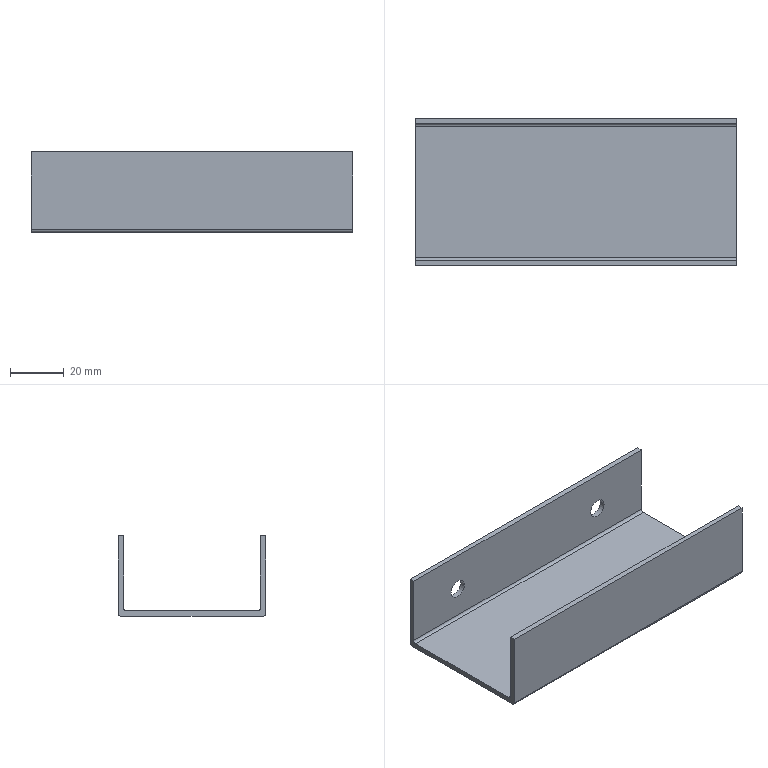Part | STEP file | 09-33 Motor support plate | 1 solid | 18 faces | box 120 x 55 x 30 mm | volume 26486 mm3 | plane 10 | cylinder 8 | commonest cylinder face diameters 2 x4 7 x4
STEP:
#1=CARTESIAN_POINT('',(0.,0.,0.));
#2=DIRECTION('',(0.,0.,1.));
#3=DIRECTION('',(1.,0.,0.));
#4=AXIS2_PLACEMENT_3D('',#1,#2,#3);
#5=CARTESIAN_POINT('',(33.27,53.,15.));
#6=VERTEX_POINT('',#5);
#7=CARTESIAN_POINT('',(33.27,55.,15.));
#8=VERTEX_POINT('',#7);
#9=CARTESIAN_POINT('',(33.27,53.,15.));
#10=DIRECTION('',(0.,1.,0.));
#11=VECTOR('',#10,1.);
#12=LINE('',#9,#11);
#13=CARTESIAN_POINT('',(36.77,53.,15.));
#14=DIRECTION('',(0.,1.,0.));
#15=DIRECTION('',(-1.,0.,0.));
#16=AXIS2_PLACEMENT_3D('',#13,#14,#15);
#17=CYLINDRICAL_SURFACE('',#16,3.5);
#18=CARTESIAN_POINT('',(6.283,0.));
#19=DIRECTION('',(0.,1.));
#20=VECTOR('',#19,1.);
#21=LINE('',#18,#20);
#22=(GEOMETRIC_REPRESENTATION_CONTEXT(2)PARAMETRIC_REPRESENTATION_CONTEXT()REPRESENTATION_CONTEXT('',''));
#23=DEFINITIONAL_REPRESENTATION('',(#21),#22);
#24=PCURVE('',#17,#23);
#25=CARTESIAN_POINT('',(36.77,53.,15.));
#26=DIRECTION('',(0.,1.,0.));
#27=DIRECTION('',(-1.,0.,0.));
#28=AXIS2_PLACEMENT_3D('',#25,#26,#27);
#29=CYLINDRICAL_SURFACE('',#28,3.5);
#30=CARTESIAN_POINT('',(0.,0.));
#31=DIRECTION('',(0.,1.));
#32=VECTOR('',#31,1.);
#33=LINE('',#30,#32);
#34=(GEOMETRIC_REPRESENTATION_CONTEXT(2)PARAMETRIC_REPRESENTATION_CONTEXT()REPRESENTATION_CONTEXT('',''));
#35=DEFINITIONAL_REPRESENTATION('',(#33),#34);
#36=PCURVE('',#29,#35);
#37=SURFACE_CURVE('',#12,(#24,#36),.PCURVE_S1.);
#38=EDGE_CURVE('',#6,#8,#37,.T.);
#39=ORIENTED_EDGE('',*,*,#38,.T.);
#40=CARTESIAN_POINT('',(40.27,55.,15.));
#41=VERTEX_POINT('',#40);
#42=CARTESIAN_POINT('',(36.77,55.,15.));
#43=DIRECTION('',(0.,1.,0.));
#44=DIRECTION('',(-1.,0.,0.));
#45=AXIS2_PLACEMENT_3D('',#42,#43,#44);
#46=CIRCLE('',#45,3.5);
#47=CARTESIAN_POINT('',(0.,2.));
#48=DIRECTION('',(1.,0.));
#49=VECTOR('',#48,1.);
#50=LINE('',#47,#49);
#51=(GEOMETRIC_REPRESENTATION_CONTEXT(2)PARAMETRIC_REPRESENTATION_CONTEXT()REPRESENTATION_CONTEXT('',''));
#52=DEFINITIONAL_REPRESENTATION('',(#50),#51);
#53=PCURVE('',#17,#52);
#54=CARTESIAN_POINT('',(-60.,55.,30.));
#55=DIRECTION('',(0.,-1.,0.));
#56=DIRECTION('',(0.,0.,-1.));
#57=AXIS2_PLACEMENT_3D('',#54,#55,#56);
#58=PLANE('',#57);
#59=CARTESIAN_POINT('',(15.,93.27));
#60=CARTESIAN_POINT('',(8.938,93.27));
#61=CARTESIAN_POINT('',(11.969,98.52));
#62=CARTESIAN_POINT('',(15.,103.77));
#63=CARTESIAN_POINT('',(18.031,98.52));
#64=CARTESIAN_POINT('',(21.062,93.27));
#65=CARTESIAN_POINT('',(15.,93.27));
#66=(BOUNDED_CURVE()B_SPLINE_CURVE(2,(#59,#60,#61,#62,#63,#64,#65),.UNSPECIFIED.,.T.,.F.)B_SPLINE_CURVE_WITH_KNOTS((1,2,2,2,2,1),(-2.094,0.,2.094,4.189,6.283,8.378),.UNSPECIFIED.)CURVE()GEOMETRIC_REPRESENTATION_ITEM()RATIONAL_B_SPLINE_CURVE((1.,0.5,1.,0.5,1.,0.5,1.))REPRESENTATION_ITEM(''));
#67=(GEOMETRIC_REPRESENTATION_CONTEXT(2)PARAMETRIC_REPRESENTATION_CONTEXT()REPRESENTATION_CONTEXT('',''));
#68=DEFINITIONAL_REPRESENTATION('',(#66),#67);
#69=PCURVE('',#58,#68);
#70=SURFACE_CURVE('',#46,(#53,#69),.PCURVE_S1.);
#71=EDGE_CURVE('',#41,#8,#70,.T.);
#72=ORIENTED_EDGE('',*,*,#71,.F.);
#73=CARTESIAN_POINT('',(40.27,53.,15.));
#74=VERTEX_POINT('',#73);
#75=CARTESIAN_POINT('',(40.27,53.,15.));
#76=DIRECTION('',(0.,1.,0.));
#77=VECTOR('',#76,1.);
#78=LINE('',#75,#77);
#79=CARTESIAN_POINT('',(3.142,0.));
#80=DIRECTION('',(0.,1.));
#81=VECTOR('',#80,1.);
#82=LINE('',#79,#81);
#83=(GEOMETRIC_REPRESENTATION_CONTEXT(2)PARAMETRIC_REPRESENTATION_CONTEXT()REPRESENTATION_CONTEXT('',''));
#84=DEFINITIONAL_REPRESENTATION('',(#82),#83);
#85=PCURVE('',#17,#84);
#86=CARTESIAN_POINT('',(3.142,0.));
#87=DIRECTION('',(0.,1.));
#88=VECTOR('',#87,1.);
#89=LINE('',#86,#88);
#90=(GEOMETRIC_REPRESENTATION_CONTEXT(2)PARAMETRIC_REPRESENTATION_CONTEXT()REPRESENTATION_CONTEXT('',''));
#91=DEFINITIONAL_REPRESENTATION('',(#89),#90);
#92=PCURVE('',#29,#91);
#93=SURFACE_CURVE('',#78,(#85,#92),.PCURVE_S1.);
#94=EDGE_CURVE('',#74,#41,#93,.T.);
#95=ORIENTED_EDGE('',*,*,#94,.F.);
#96=CARTESIAN_POINT('',(36.77,53.,15.));
#97=DIRECTION('',(0.,-1.,0.));
#98=DIRECTION('',(-1.,0.,0.));
#99=AXIS2_PLACEMENT_3D('',#96,#97,#98);
#100=CIRCLE('',#99,3.5);
#101=CARTESIAN_POINT('',(6.283,0.));
#102=DIRECTION('',(-1.,0.));
#103=VECTOR('',#102,1.);
#104=LINE('',#101,#103);
#105=(GEOMETRIC_REPRESENTATION_CONTEXT(2)PARAMETRIC_REPRESENTATION_CONTEXT()REPRESENTATION_CONTEXT('',''));
#106=DEFINITIONAL_REPRESENTATION('',(#104),#105);
#107=PCURVE('',#17,#106);
#108=CARTESIAN_POINT('',(-60.,53.,3.));
#109=DIRECTION('',(0.,1.,0.));
#110=DIRECTION('',(0.,0.,1.));
#111=AXIS2_PLACEMENT_3D('',#108,#109,#110);
#112=PLANE('',#111);
#113=CARTESIAN_POINT('',(12.,93.27));
#114=CARTESIAN_POINT('',(5.938,93.27));
#115=CARTESIAN_POINT('',(8.969,98.52));
#116=CARTESIAN_POINT('',(12.,103.77));
#117=CARTESIAN_POINT('',(15.031,98.52));
#118=CARTESIAN_POINT('',(18.062,93.27));
#119=CARTESIAN_POINT('',(12.,93.27));
#120=(BOUNDED_CURVE()B_SPLINE_CURVE(2,(#113,#114,#115,#116,#117,#118,#119),.UNSPECIFIED.,.T.,.F.)B_SPLINE_CURVE_WITH_KNOTS((1,2,2,2,2,1),(-2.094,0.,2.094,4.189,6.283,8.378),.UNSPECIFIED.)CURVE()GEOMETRIC_REPRESENTATION_ITEM()RATIONAL_B_SPLINE_CURVE((1.,0.5,1.,0.5,1.,0.5,1.))REPRESENTATION_ITEM(''));
#121=(GEOMETRIC_REPRESENTATION_CONTEXT(2)PARAMETRIC_REPRESENTATION_CONTEXT()REPRESENTATION_CONTEXT('',''));
#122=DEFINITIONAL_REPRESENTATION('',(#120),#121);
#123=PCURVE('',#112,#122);
#124=SURFACE_CURVE('',#100,(#107,#123),.PCURVE_S1.);
#125=EDGE_CURVE('',#6,#74,#124,.T.);
#126=ORIENTED_EDGE('',*,*,#125,.F.);
#127=EDGE_LOOP('',(#39,#72,#95,#126));
#128=FACE_BOUND('',#127,.F.);
#129=ADVANCED_FACE('',(#128),#17,.F.);
#130=CARTESIAN_POINT('',(-40.27,53.,15.));
#131=VERTEX_POINT('',#130);
#132=CARTESIAN_POINT('',(-40.27,55.,15.));
#133=VERTEX_POINT('',#132);
#134=CARTESIAN_POINT('',(-40.27,53.,15.));
#135=DIRECTION('',(0.,1.,0.));
#136=VECTOR('',#135,1.);
#137=LINE('',#134,#136);
#138=CARTESIAN_POINT('',(-36.77,53.,15.));
#139=DIRECTION('',(0.,1.,0.));
#140=DIRECTION('',(-1.,0.,0.));
#141=AXIS2_PLACEMENT_3D('',#138,#139,#140);
#142=CYLINDRICAL_SURFACE('',#141,3.5);
#143=CARTESIAN_POINT('',(6.283,0.));
#144=DIRECTION('',(0.,1.));
#145=VECTOR('',#144,1.);
#146=LINE('',#143,#145);
#147=(GEOMETRIC_REPRESENTATION_CONTEXT(2)PARAMETRIC_REPRESENTATION_CONTEXT()REPRESENTATION_CONTEXT('',''));
#148=DEFINITIONAL_REPRESENTATION('',(#146),#147);
#149=PCURVE('',#142,#148);
#150=CARTESIAN_POINT('',(-36.77,53.,15.));
#151=DIRECTION('',(0.,1.,0.));
#152=DIRECTION('',(-1.,0.,0.));
#153=AXIS2_PLACEMENT_3D('',#150,#151,#152);
#154=CYLINDRICAL_SURFACE('',#153,3.5);
#155=CARTESIAN_POINT('',(0.,0.));
#156=DIRECTION('',(0.,1.));
#157=VECTOR('',#156,1.);
#158=LINE('',#155,#157);
#159=(GEOMETRIC_REPRESENTATION_CONTEXT(2)PARAMETRIC_REPRESENTATION_CONTEXT()REPRESENTATION_CONTEXT('',''));
#160=DEFINITIONAL_REPRESENTATION('',(#158),#159);
#161=PCURVE('',#154,#160);
#162=SURFACE_CURVE('',#137,(#149,#161),.PCURVE_S1.);
#163=EDGE_CURVE('',#131,#133,#162,.T.);
#164=ORIENTED_EDGE('',*,*,#163,.T.);
#165=CARTESIAN_POINT('',(-33.27,55.,15.));
#166=VERTEX_POINT('',#165);
#167=CARTESIAN_POINT('',(-36.77,55.,15.));
#168=DIRECTION('',(0.,1.,0.));
#169=DIRECTION('',(-1.,0.,0.));
#170=AXIS2_PLACEMENT_3D('',#167,#168,#169);
#171=CIRCLE('',#170,3.5);
#172=CARTESIAN_POINT('',(0.,2.));
#173=DIRECTION('',(1.,0.));
#174=VECTOR('',#173,1.);
#175=LINE('',#172,#174);
#176=(GEOMETRIC_REPRESENTATION_CONTEXT(2)PARAMETRIC_REPRESENTATION_CONTEXT()REPRESENTATION_CONTEXT('',''));
#177=DEFINITIONAL_REPRESENTATION('',(#175),#176);
#178=PCURVE('',#142,#177);
#179=CARTESIAN_POINT('',(15.,19.73));
#180=CARTESIAN_POINT('',(8.938,19.73));
#181=CARTESIAN_POINT('',(11.969,24.98));
#182=CARTESIAN_POINT('',(15.,30.23));
#183=CARTESIAN_POINT('',(18.031,24.98));
#184=CARTESIAN_POINT('',(21.062,19.73));
#185=CARTESIAN_POINT('',(15.,19.73));
#186=(BOUNDED_CURVE()B_SPLINE_CURVE(2,(#179,#180,#181,#182,#183,#184,#185),.UNSPECIFIED.,.T.,.F.)B_SPLINE_CURVE_WITH_KNOTS((1,2,2,2,2,1),(-2.094,0.,2.094,4.189,6.283,8.378),.UNSPECIFIED.)CURVE()GEOMETRIC_REPRESENTATION_ITEM()RATIONAL_B_SPLINE_CURVE((1.,0.5,1.,0.5,1.,0.5,1.))REPRESENTATION_ITEM(''));
#187=(GEOMETRIC_REPRESENTATION_CONTEXT(2)PARAMETRIC_REPRESENTATION_CONTEXT()REPRESENTATION_CONTEXT('',''));
#188=DEFINITIONAL_REPRESENTATION('',(#186),#187);
#189=PCURVE('',#58,#188);
#190=SURFACE_CURVE('',#171,(#178,#189),.PCURVE_S1.);
#191=EDGE_CURVE('',#166,#133,#190,.T.);
#192=ORIENTED_EDGE('',*,*,#191,.F.);
#193=CARTESIAN_POINT('',(-33.27,53.,15.));
#194=VERTEX_POINT('',#193);
#195=CARTESIAN_POINT('',(-33.27,53.,15.));
#196=DIRECTION('',(0.,1.,0.));
#197=VECTOR('',#196,1.);
#198=LINE('',#195,#197);
#199=CARTESIAN_POINT('',(3.142,0.));
#200=DIRECTION('',(0.,1.));
#201=VECTOR('',#200,1.);
#202=LINE('',#199,#201);
#203=(GEOMETRIC_REPRESENTATION_CONTEXT(2)PARAMETRIC_REPRESENTATION_CONTEXT()REPRESENTATION_CONTEXT('',''));
#204=DEFINITIONAL_REPRESENTATION('',(#202),#203);
#205=PCURVE('',#142,#204);
#206=CARTESIAN_POINT('',(3.142,0.));
#207=DIRECTION('',(0.,1.));
#208=VECTOR('',#207,1.);
#209=LINE('',#206,#208);
#210=(GEOMETRIC_REPRESENTATION_CONTEXT(2)PARAMETRIC_REPRESENTATION_CONTEXT()REPRESENTATION_CONTEXT('',''));
#211=DEFINITIONAL_REPRESENTATION('',(#209),#210);
#212=PCURVE('',#154,#211);
#213=SURFACE_CURVE('',#198,(#205,#212),.PCURVE_S1.);
#214=EDGE_CURVE('',#194,#166,#213,.T.);
#215=ORIENTED_EDGE('',*,*,#214,.F.);
#216=CARTESIAN_POINT('',(-36.77,53.,15.));
#217=DIRECTION('',(0.,-1.,0.));
#218=DIRECTION('',(-1.,0.,0.));
#219=AXIS2_PLACEMENT_3D('',#216,#217,#218);
#220=CIRCLE('',#219,3.5);
#221=CARTESIAN_POINT('',(6.283,0.));
#222=DIRECTION('',(-1.,0.));
#223=VECTOR('',#222,1.);
#224=LINE('',#221,#223);
#225=(GEOMETRIC_REPRESENTATION_CONTEXT(2)PARAMETRIC_REPRESENTATION_CONTEXT()REPRESENTATION_CONTEXT('',''));
#226=DEFINITIONAL_REPRESENTATION('',(#224),#225);
#227=PCURVE('',#142,#226);
#228=CARTESIAN_POINT('',(12.,19.73));
#229=CARTESIAN_POINT('',(5.938,19.73));
#230=CARTESIAN_POINT('',(8.969,24.98));
#231=CARTESIAN_POINT('',(12.,30.23));
#232=CARTESIAN_POINT('',(15.031,24.98));
#233=CARTESIAN_POINT('',(18.062,19.73));
#234=CARTESIAN_POINT('',(12.,19.73));
#235=(BOUNDED_CURVE()B_SPLINE_CURVE(2,(#228,#229,#230,#231,#232,#233,#234),.UNSPECIFIED.,.T.,.F.)B_SPLINE_CURVE_WITH_KNOTS((1,2,2,2,2,1),(-2.094,0.,2.094,4.189,6.283,8.378),.UNSPECIFIED.)CURVE()GEOMETRIC_REPRESENTATION_ITEM()RATIONAL_B_SPLINE_CURVE((1.,0.5,1.,0.5,1.,0.5,1.))REPRESENTATION_ITEM(''));
#236=(GEOMETRIC_REPRESENTATION_CONTEXT(2)PARAMETRIC_REPRESENTATION_CONTEXT()REPRESENTATION_CONTEXT('',''));
#237=DEFINITIONAL_REPRESENTATION('',(#235),#236);
#238=PCURVE('',#112,#237);
#239=SURFACE_CURVE('',#220,(#227,#238),.PCURVE_S1.);
#240=EDGE_CURVE('',#131,#194,#239,.T.);
#241=ORIENTED_EDGE('',*,*,#240,.F.);
#242=EDGE_LOOP('',(#164,#192,#215,#241));
#243=FACE_BOUND('',#242,.F.);
#244=ADVANCED_FACE('',(#243),#142,.F.);
#245=CARTESIAN_POINT('',(36.77,55.,15.));
#246=DIRECTION('',(0.,1.,0.));
#247=DIRECTION('',(-1.,0.,0.));
#248=AXIS2_PLACEMENT_3D('',#245,#246,#247);
#249=CIRCLE('',#248,3.5);
#250=CARTESIAN_POINT('',(0.,2.));
#251=DIRECTION('',(1.,0.));
#252=VECTOR('',#251,1.);
#253=LINE('',#250,#252);
#254=(GEOMETRIC_REPRESENTATION_CONTEXT(2)PARAMETRIC_REPRESENTATION_CONTEXT()REPRESENTATION_CONTEXT('',''));
#255=DEFINITIONAL_REPRESENTATION('',(#253),#254);
#256=PCURVE('',#29,#255);
#257=CARTESIAN_POINT('',(15.,93.27));
#258=CARTESIAN_POINT('',(8.938,93.27));
#259=CARTESIAN_POINT('',(11.969,98.52));
#260=CARTESIAN_POINT('',(15.,103.77));
#261=CARTESIAN_POINT('',(18.031,98.52));
#262=CARTESIAN_POINT('',(21.062,93.27));
#263=CARTESIAN_POINT('',(15.,93.27));
#264=(BOUNDED_CURVE()B_SPLINE_CURVE(2,(#257,#258,#259,#260,#261,#262,#263),.UNSPECIFIED.,.T.,.F.)B_SPLINE_CURVE_WITH_KNOTS((1,2,2,2,2,1),(-2.094,0.,2.094,4.189,6.283,8.378),.UNSPECIFIED.)CURVE()GEOMETRIC_REPRESENTATION_ITEM()RATIONAL_B_SPLINE_CURVE((1.,0.5,1.,0.5,1.,0.5,1.))REPRESENTATION_ITEM(''));
#265=(GEOMETRIC_REPRESENTATION_CONTEXT(2)PARAMETRIC_REPRESENTATION_CONTEXT()REPRESENTATION_CONTEXT('',''));
#266=DEFINITIONAL_REPRESENTATION('',(#264),#265);
#267=PCURVE('',#58,#266);
#268=SURFACE_CURVE('',#249,(#256,#267),.PCURVE_S1.);
#269=EDGE_CURVE('',#8,#41,#268,.T.);
#270=ORIENTED_EDGE('',*,*,#269,.F.);
#271=ORIENTED_EDGE('',*,*,#38,.F.);
#272=CARTESIAN_POINT('',(36.77,53.,15.));
#273=DIRECTION('',(0.,-1.,0.));
#274=DIRECTION('',(-1.,0.,0.));
#275=AXIS2_PLACEMENT_3D('',#272,#273,#274);
#276=CIRCLE('',#275,3.5);
#277=CARTESIAN_POINT('',(6.283,0.));
#278=DIRECTION('',(-1.,0.));
#279=VECTOR('',#278,1.);
#280=LINE('',#277,#279);
#281=(GEOMETRIC_REPRESENTATION_CONTEXT(2)PARAMETRIC_REPRESENTATION_CONTEXT()REPRESENTATION_CONTEXT('',''));
#282=DEFINITIONAL_REPRESENTATION('',(#280),#281);
#283=PCURVE('',#29,#282);
#284=CARTESIAN_POINT('',(12.,93.27));
#285=CARTESIAN_POINT('',(5.938,93.27));
#286=CARTESIAN_POINT('',(8.969,98.52));
#287=CARTESIAN_POINT('',(12.,103.77));
#288=CARTESIAN_POINT('',(15.031,98.52));
#289=CARTESIAN_POINT('',(18.062,93.27));
#290=CARTESIAN_POINT('',(12.,93.27));
#291=(BOUNDED_CURVE()B_SPLINE_CURVE(2,(#284,#285,#286,#287,#288,#289,#290),.UNSPECIFIED.,.T.,.F.)B_SPLINE_CURVE_WITH_KNOTS((1,2,2,2,2,1),(-2.094,0.,2.094,4.189,6.283,8.378),.UNSPECIFIED.)CURVE()GEOMETRIC_REPRESENTATION_ITEM()RATIONAL_B_SPLINE_CURVE((1.,0.5,1.,0.5,1.,0.5,1.))REPRESENTATION_ITEM(''));
#292=(GEOMETRIC_REPRESENTATION_CONTEXT(2)PARAMETRIC_REPRESENTATION_CONTEXT()REPRESENTATION_CONTEXT('',''));
#293=DEFINITIONAL_REPRESENTATION('',(#291),#292);
#294=PCURVE('',#112,#293);
#295=SURFACE_CURVE('',#276,(#283,#294),.PCURVE_S1.);
#296=EDGE_CURVE('',#74,#6,#295,.T.);
#297=ORIENTED_EDGE('',*,*,#296,.F.);
#298=ORIENTED_EDGE('',*,*,#94,.T.);
#299=EDGE_LOOP('',(#270,#271,#297,#298));
#300=FACE_BOUND('',#299,.F.);
#301=ADVANCED_FACE('',(#300),#29,.F.);
#302=CARTESIAN_POINT('',(-36.77,55.,15.));
#303=DIRECTION('',(0.,1.,0.));
#304=DIRECTION('',(-1.,0.,0.));
#305=AXIS2_PLACEMENT_3D('',#302,#303,#304);
#306=CIRCLE('',#305,3.5);
#307=CARTESIAN_POINT('',(15.,19.73));
#308=CARTESIAN_POINT('',(8.938,19.73));
#309=CARTESIAN_POINT('',(11.969,24.98));
#310=CARTESIAN_POINT('',(15.,30.23));
#311=CARTESIAN_POINT('',(18.031,24.98));
#312=CARTESIAN_POINT('',(21.062,19.73));
#313=CARTESIAN_POINT('',(15.,19.73));
#314=(BOUNDED_CURVE()B_SPLINE_CURVE(2,(#307,#308,#309,#310,#311,#312,#313),.UNSPECIFIED.,.T.,.F.)B_SPLINE_CURVE_WITH_KNOTS((1,2,2,2,2,1),(-2.094,0.,2.094,4.189,6.283,8.378),.UNSPECIFIED.)CURVE()GEOMETRIC_REPRESENTATION_ITEM()RATIONAL_B_SPLINE_CURVE((1.,0.5,1.,0.5,1.,0.5,1.))REPRESENTATION_ITEM(''));
#315=(GEOMETRIC_REPRESENTATION_CONTEXT(2)PARAMETRIC_REPRESENTATION_CONTEXT()REPRESENTATION_CONTEXT('',''));
#316=DEFINITIONAL_REPRESENTATION('',(#314),#315);
#317=PCURVE('',#58,#316);
#318=CARTESIAN_POINT('',(0.,2.));
#319=DIRECTION('',(1.,0.));
#320=VECTOR('',#319,1.);
#321=LINE('',#318,#320);
#322=(GEOMETRIC_REPRESENTATION_CONTEXT(2)PARAMETRIC_REPRESENTATION_CONTEXT()REPRESENTATION_CONTEXT('',''));
#323=DEFINITIONAL_REPRESENTATION('',(#321),#322);
#324=PCURVE('',#154,#323);
#325=SURFACE_CURVE('',#306,(#317,#324),.PCURVE_S1.);
#326=EDGE_CURVE('',#133,#166,#325,.T.);
#327=ORIENTED_EDGE('',*,*,#326,.F.);
#328=ORIENTED_EDGE('',*,*,#191,.F.);
#329=EDGE_LOOP('',(#327,#328));
#330=FACE_BOUND('',#329,.T.);
#331=ORIENTED_EDGE('',*,*,#269,.F.);
#332=ORIENTED_EDGE('',*,*,#71,.F.);
#333=EDGE_LOOP('',(#331,#332));
#334=FACE_BOUND('',#333,.T.);
#335=CARTESIAN_POINT('',(-60.,55.,1.));
#336=VERTEX_POINT('',#335);
#337=CARTESIAN_POINT('',(60.,55.,1.));
#338=VERTEX_POINT('',#337);
#339=CARTESIAN_POINT('',(0.,55.,1.));
#340=DIRECTION('',(1.,0.,0.));
#341=VECTOR('',#340,1.);
#342=LINE('',#339,#341);
#343=CARTESIAN_POINT('',(29.,60.));
#344=DIRECTION('',(0.,1.));
#345=VECTOR('',#344,1.);
#346=LINE('',#343,#345);
#347=(GEOMETRIC_REPRESENTATION_CONTEXT(2)PARAMETRIC_REPRESENTATION_CONTEXT()REPRESENTATION_CONTEXT('',''));
#348=DEFINITIONAL_REPRESENTATION('',(#346),#347);
#349=PCURVE('',#58,#348);
#350=CARTESIAN_POINT('',(60.,54.,1.));
#351=DIRECTION('',(-1.,0.,0.));
#352=DIRECTION('',(0.,-1.,0.));
#353=AXIS2_PLACEMENT_3D('',#350,#351,#352);
#354=CYLINDRICAL_SURFACE('',#353,1.);
#355=CARTESIAN_POINT('',(3.142,60.));
#356=DIRECTION('',(0.,-1.));
#357=VECTOR('',#356,1.);
#358=LINE('',#355,#357);
#359=(GEOMETRIC_REPRESENTATION_CONTEXT(2)PARAMETRIC_REPRESENTATION_CONTEXT()REPRESENTATION_CONTEXT('',''));
#360=DEFINITIONAL_REPRESENTATION('',(#358),#359);
#361=PCURVE('',#354,#360);
#362=SURFACE_CURVE('',#342,(#349,#361),.PCURVE_S1.);
#363=EDGE_CURVE('',#336,#338,#362,.T.);
#364=ORIENTED_EDGE('',*,*,#363,.F.);
#365=CARTESIAN_POINT('',(-60.,55.,30.));
#366=VERTEX_POINT('',#365);
#367=CARTESIAN_POINT('',(-60.,55.,15.5));
#368=DIRECTION('',(0.,0.,-1.));
#369=VECTOR('',#368,1.);
#370=LINE('',#367,#369);
#371=CARTESIAN_POINT('',(14.5,0.));
#372=DIRECTION('',(1.,0.));
#373=VECTOR('',#372,1.);
#374=LINE('',#371,#373);
#375=(GEOMETRIC_REPRESENTATION_CONTEXT(2)PARAMETRIC_REPRESENTATION_CONTEXT()REPRESENTATION_CONTEXT('',''));
#376=DEFINITIONAL_REPRESENTATION('',(#374),#375);
#377=PCURVE('',#58,#376);
#378=CARTESIAN_POINT('',(-60.,0.,30.));
#379=DIRECTION('',(1.,0.,0.));
#380=DIRECTION('',(0.,0.,-1.));
#381=AXIS2_PLACEMENT_3D('',#378,#379,#380);
#382=PLANE('',#381);
#383=CARTESIAN_POINT('',(14.5,55.));
#384=DIRECTION('',(1.,0.));
#385=VECTOR('',#384,1.);
#386=LINE('',#383,#385);
#387=(GEOMETRIC_REPRESENTATION_CONTEXT(2)PARAMETRIC_REPRESENTATION_CONTEXT()REPRESENTATION_CONTEXT('',''));
#388=DEFINITIONAL_REPRESENTATION('',(#386),#387);
#389=PCURVE('',#382,#388);
#390=SURFACE_CURVE('',#370,(#377,#389),.PCURVE_S1.);
#391=EDGE_CURVE('',#366,#336,#390,.T.);
#392=ORIENTED_EDGE('',*,*,#391,.F.);
#393=CARTESIAN_POINT('',(60.,55.,30.));
#394=VERTEX_POINT('',#393);
#395=CARTESIAN_POINT('',(0.,55.,30.));
#396=DIRECTION('',(-1.,0.,0.));
#397=VECTOR('',#396,1.);
#398=LINE('',#395,#397);
#399=CARTESIAN_POINT('',(0.,60.));
#400=DIRECTION('',(0.,-1.));
#401=VECTOR('',#400,1.);
#402=LINE('',#399,#401);
#403=(GEOMETRIC_REPRESENTATION_CONTEXT(2)PARAMETRIC_REPRESENTATION_CONTEXT()REPRESENTATION_CONTEXT('',''));
#404=DEFINITIONAL_REPRESENTATION('',(#402),#403);
#405=PCURVE('',#58,#404);
#406=CARTESIAN_POINT('',(60.,53.,30.));
#407=DIRECTION('',(0.,0.,-1.));
#408=DIRECTION('',(-1.,0.,0.));
#409=AXIS2_PLACEMENT_3D('',#406,#407,#408);
#410=PLANE('',#409);
#411=CARTESIAN_POINT('',(60.,2.));
#412=DIRECTION('',(1.,0.));
#413=VECTOR('',#412,1.);
#414=LINE('',#411,#413);
#415=(GEOMETRIC_REPRESENTATION_CONTEXT(2)PARAMETRIC_REPRESENTATION_CONTEXT()REPRESENTATION_CONTEXT('',''));
#416=DEFINITIONAL_REPRESENTATION('',(#414),#415);
#417=PCURVE('',#410,#416);
#418=SURFACE_CURVE('',#398,(#405,#417),.PCURVE_S1.);
#419=EDGE_CURVE('',#394,#366,#418,.T.);
#420=ORIENTED_EDGE('',*,*,#419,.F.);
#421=CARTESIAN_POINT('',(60.,55.,15.5));
#422=DIRECTION('',(0.,0.,1.));
#423=VECTOR('',#422,1.);
#424=LINE('',#421,#423);
#425=CARTESIAN_POINT('',(14.5,120.));
#426=DIRECTION('',(-1.,0.));
#427=VECTOR('',#426,1.);
#428=LINE('',#425,#427);
#429=(GEOMETRIC_REPRESENTATION_CONTEXT(2)PARAMETRIC_REPRESENTATION_CONTEXT()REPRESENTATION_CONTEXT('',''));
#430=DEFINITIONAL_REPRESENTATION('',(#428),#429);
#431=PCURVE('',#58,#430);
#432=CARTESIAN_POINT('',(60.,0.,30.));
#433=DIRECTION('',(1.,0.,0.));
#434=DIRECTION('',(0.,0.,-1.));
#435=AXIS2_PLACEMENT_3D('',#432,#433,#434);
#436=PLANE('',#435);
#437=CARTESIAN_POINT('',(14.5,55.));
#438=DIRECTION('',(-1.,0.));
#439=VECTOR('',#438,1.);
#440=LINE('',#437,#439);
#441=(GEOMETRIC_REPRESENTATION_CONTEXT(2)PARAMETRIC_REPRESENTATION_CONTEXT()REPRESENTATION_CONTEXT('',''));
#442=DEFINITIONAL_REPRESENTATION('',(#440),#441);
#443=PCURVE('',#436,#442);
#444=SURFACE_CURVE('',#424,(#431,#443),.PCURVE_S1.);
#445=EDGE_CURVE('',#338,#394,#444,.T.);
#446=ORIENTED_EDGE('',*,*,#445,.F.);
#447=EDGE_LOOP('',(#364,#392,#420,#446));
#448=FACE_BOUND('',#447,.T.);
#449=ADVANCED_FACE('',(#330,#334,#448),#58,.F.);
#450=ORIENTED_EDGE('',*,*,#240,.F.);
#451=CARTESIAN_POINT('',(-36.77,53.,15.));
#452=DIRECTION('',(0.,-1.,0.));
#453=DIRECTION('',(-1.,0.,0.));
#454=AXIS2_PLACEMENT_3D('',#451,#452,#453);
#455=CIRCLE('',#454,3.5);
#456=CARTESIAN_POINT('',(12.,19.73));
#457=CARTESIAN_POINT('',(5.938,19.73));
#458=CARTESIAN_POINT('',(8.969,24.98));
#459=CARTESIAN_POINT('',(12.,30.23));
#460=CARTESIAN_POINT('',(15.031,24.98));
#461=CARTESIAN_POINT('',(18.062,19.73));
#462=CARTESIAN_POINT('',(12.,19.73));
#463=(BOUNDED_CURVE()B_SPLINE_CURVE(2,(#456,#457,#458,#459,#460,#461,#462),.UNSPECIFIED.,.T.,.F.)B_SPLINE_CURVE_WITH_KNOTS((1,2,2,2,2,1),(-2.094,0.,2.094,4.189,6.283,8.378),.UNSPECIFIED.)CURVE()GEOMETRIC_REPRESENTATION_ITEM()RATIONAL_B_SPLINE_CURVE((1.,0.5,1.,0.5,1.,0.5,1.))REPRESENTATION_ITEM(''));
#464=(GEOMETRIC_REPRESENTATION_CONTEXT(2)PARAMETRIC_REPRESENTATION_CONTEXT()REPRESENTATION_CONTEXT('',''));
#465=DEFINITIONAL_REPRESENTATION('',(#463),#464);
#466=PCURVE('',#112,#465);
#467=CARTESIAN_POINT('',(6.283,0.));
#468=DIRECTION('',(-1.,0.));
#469=VECTOR('',#468,1.);
#470=LINE('',#467,#469);
#471=(GEOMETRIC_REPRESENTATION_CONTEXT(2)PARAMETRIC_REPRESENTATION_CONTEXT()REPRESENTATION_CONTEXT('',''));
#472=DEFINITIONAL_REPRESENTATION('',(#470),#471);
#473=PCURVE('',#154,#472);
#474=SURFACE_CURVE('',#455,(#466,#473),.PCURVE_S1.);
#475=EDGE_CURVE('',#194,#131,#474,.T.);
#476=ORIENTED_EDGE('',*,*,#475,.F.);
#477=EDGE_LOOP('',(#450,#476));
#478=FACE_BOUND('',#477,.T.);
#479=ORIENTED_EDGE('',*,*,#125,.F.);
#480=ORIENTED_EDGE('',*,*,#296,.F.);
#481=EDGE_LOOP('',(#479,#480));
#482=FACE_BOUND('',#481,.T.);
#483=CARTESIAN_POINT('',(60.,53.,3.));
#484=VERTEX_POINT('',#483);
#485=CARTESIAN_POINT('',(-60.,53.,3.));
#486=VERTEX_POINT('',#485);
#487=CARTESIAN_POINT('',(0.,53.,3.));
#488=DIRECTION('',(-1.,0.,0.));
#489=VECTOR('',#488,1.);
#490=LINE('',#487,#489);
#491=CARTESIAN_POINT('',(0.,60.));
#492=DIRECTION('',(0.,-1.));
#493=VECTOR('',#492,1.);
#494=LINE('',#491,#493);
#495=(GEOMETRIC_REPRESENTATION_CONTEXT(2)PARAMETRIC_REPRESENTATION_CONTEXT()REPRESENTATION_CONTEXT('',''));
#496=DEFINITIONAL_REPRESENTATION('',(#494),#495);
#497=PCURVE('',#112,#496);
#498=CARTESIAN_POINT('',(-60.,52.,3.));
#499=DIRECTION('',(1.,0.,0.));
#500=DIRECTION('',(0.,1.,0.));
#501=AXIS2_PLACEMENT_3D('',#498,#499,#500);
#502=CYLINDRICAL_SURFACE('',#501,1.);
#503=CARTESIAN_POINT('',(6.283,60.));
#504=DIRECTION('',(0.,-1.));
#505=VECTOR('',#504,1.);
#506=LINE('',#503,#505);
#507=(GEOMETRIC_REPRESENTATION_CONTEXT(2)PARAMETRIC_REPRESENTATION_CONTEXT()REPRESENTATION_CONTEXT('',''));
#508=DEFINITIONAL_REPRESENTATION('',(#506),#507);
#509=PCURVE('',#502,#508);
#510=SURFACE_CURVE('',#490,(#497,#509),.PCURVE_S1.);
#511=EDGE_CURVE('',#484,#486,#510,.T.);
#512=ORIENTED_EDGE('',*,*,#511,.F.);
#513=CARTESIAN_POINT('',(60.,53.,30.));
#514=VERTEX_POINT('',#513);
#515=CARTESIAN_POINT('',(60.,53.,16.5));
#516=DIRECTION('',(0.,0.,-1.));
#517=VECTOR('',#516,1.);
#518=LINE('',#515,#517);
#519=CARTESIAN_POINT('',(13.5,120.));
#520=DIRECTION('',(-1.,0.));
#521=VECTOR('',#520,1.);
#522=LINE('',#519,#521);
#523=(GEOMETRIC_REPRESENTATION_CONTEXT(2)PARAMETRIC_REPRESENTATION_CONTEXT()REPRESENTATION_CONTEXT('',''));
#524=DEFINITIONAL_REPRESENTATION('',(#522),#523);
#525=PCURVE('',#112,#524);
#526=CARTESIAN_POINT('',(13.5,53.));
#527=DIRECTION('',(1.,0.));
#528=VECTOR('',#527,1.);
#529=LINE('',#526,#528);
#530=(GEOMETRIC_REPRESENTATION_CONTEXT(2)PARAMETRIC_REPRESENTATION_CONTEXT()REPRESENTATION_CONTEXT('',''));
#531=DEFINITIONAL_REPRESENTATION('',(#529),#530);
#532=PCURVE('',#436,#531);
#533=SURFACE_CURVE('',#518,(#525,#532),.PCURVE_S1.);
#534=EDGE_CURVE('',#514,#484,#533,.T.);
#535=ORIENTED_EDGE('',*,*,#534,.F.);
#536=CARTESIAN_POINT('',(-60.,53.,30.));
#537=VERTEX_POINT('',#536);
#538=CARTESIAN_POINT('',(0.,53.,30.));
#539=DIRECTION('',(1.,0.,0.));
#540=VECTOR('',#539,1.);
#541=LINE('',#538,#540);
#542=CARTESIAN_POINT('',(27.,60.));
#543=DIRECTION('',(0.,1.));
#544=VECTOR('',#543,1.);
#545=LINE('',#542,#544);
#546=(GEOMETRIC_REPRESENTATION_CONTEXT(2)PARAMETRIC_REPRESENTATION_CONTEXT()REPRESENTATION_CONTEXT('',''));
#547=DEFINITIONAL_REPRESENTATION('',(#545),#546);
#548=PCURVE('',#112,#547);
#549=CARTESIAN_POINT('',(60.,0.));
#550=DIRECTION('',(-1.,0.));
#551=VECTOR('',#550,1.);
#552=LINE('',#549,#551);
#553=(GEOMETRIC_REPRESENTATION_CONTEXT(2)PARAMETRIC_REPRESENTATION_CONTEXT()REPRESENTATION_CONTEXT('',''));
#554=DEFINITIONAL_REPRESENTATION('',(#552),#553);
#555=PCURVE('',#410,#554);
#556=SURFACE_CURVE('',#541,(#548,#555),.PCURVE_S1.);
#557=EDGE_CURVE('',#537,#514,#556,.T.);
#558=ORIENTED_EDGE('',*,*,#557,.F.);
#559=CARTESIAN_POINT('',(-60.,53.,16.5));
#560=DIRECTION('',(0.,0.,1.));
#561=VECTOR('',#560,1.);
#562=LINE('',#559,#561);
#563=CARTESIAN_POINT('',(13.5,0.));
#564=DIRECTION('',(1.,0.));
#565=VECTOR('',#564,1.);
#566=LINE('',#563,#565);
#567=(GEOMETRIC_REPRESENTATION_CONTEXT(2)PARAMETRIC_REPRESENTATION_CONTEXT()REPRESENTATION_CONTEXT('',''));
#568=DEFINITIONAL_REPRESENTATION('',(#566),#567);
#569=PCURVE('',#112,#568);
#570=CARTESIAN_POINT('',(13.5,53.));
#571=DIRECTION('',(-1.,0.));
#572=VECTOR('',#571,1.);
#573=LINE('',#570,#572);
#574=(GEOMETRIC_REPRESENTATION_CONTEXT(2)PARAMETRIC_REPRESENTATION_CONTEXT()REPRESENTATION_CONTEXT('',''));
#575=DEFINITIONAL_REPRESENTATION('',(#573),#574);
#576=PCURVE('',#382,#575);
#577=SURFACE_CURVE('',#562,(#569,#576),.PCURVE_S1.);
#578=EDGE_CURVE('',#486,#537,#577,.T.);
#579=ORIENTED_EDGE('',*,*,#578,.F.);
#580=EDGE_LOOP('',(#512,#535,#558,#579));
#581=FACE_BOUND('',#580,.T.);
#582=ADVANCED_FACE('',(#478,#482,#581),#112,.F.);
#583=ORIENTED_EDGE('',*,*,#326,.F.);
#584=ORIENTED_EDGE('',*,*,#163,.F.);
#585=ORIENTED_EDGE('',*,*,#475,.F.);
#586=ORIENTED_EDGE('',*,*,#214,.T.);
#587=EDGE_LOOP('',(#583,#584,#585,#586));
#588=FACE_BOUND('',#587,.F.);
#589=ADVANCED_FACE('',(#588),#154,.F.);
#590=CARTESIAN_POINT('',(60.,0.,30.));
#591=VERTEX_POINT('',#590);
#592=CARTESIAN_POINT('',(60.,0.,1.));
#593=VERTEX_POINT('',#592);
#594=CARTESIAN_POINT('',(60.,0.,15.));
#595=DIRECTION('',(0.,0.,-1.));
#596=VECTOR('',#595,1.);
#597=LINE('',#594,#596);
#598=CARTESIAN_POINT('',(15.,0.));
#599=DIRECTION('',(1.,0.));
#600=VECTOR('',#599,1.);
#601=LINE('',#598,#600);
#602=(GEOMETRIC_REPRESENTATION_CONTEXT(2)PARAMETRIC_REPRESENTATION_CONTEXT()REPRESENTATION_CONTEXT('',''));
#603=DEFINITIONAL_REPRESENTATION('',(#601),#602);
#604=PCURVE('',#436,#603);
#605=CARTESIAN_POINT('',(-60.,0.,1.));
#606=DIRECTION('',(0.,1.,0.));
#607=DIRECTION('',(0.,0.,1.));
#608=AXIS2_PLACEMENT_3D('',#605,#606,#607);
#609=PLANE('',#608);
#610=CARTESIAN_POINT('',(14.,120.));
#611=DIRECTION('',(-1.,0.));
#612=VECTOR('',#611,1.);
#613=LINE('',#610,#612);
#614=(GEOMETRIC_REPRESENTATION_CONTEXT(2)PARAMETRIC_REPRESENTATION_CONTEXT()REPRESENTATION_CONTEXT('',''));
#615=DEFINITIONAL_REPRESENTATION('',(#613),#614);
#616=PCURVE('',#609,#615);
#617=SURFACE_CURVE('',#597,(#604,#616),.PCURVE_S1.);
#618=EDGE_CURVE('',#591,#593,#617,.T.);
#619=ORIENTED_EDGE('',*,*,#618,.T.);
#620=CARTESIAN_POINT('',(60.,1.,0.));
#621=VERTEX_POINT('',#620);
#622=CARTESIAN_POINT('',(60.,1.,1.));
#623=DIRECTION('',(1.,0.,0.));
#624=DIRECTION('',(0.,-1.,0.));
#625=AXIS2_PLACEMENT_3D('',#622,#623,#624);
#626=CIRCLE('',#625,1.);
#627=CARTESIAN_POINT('',(29.,1.));
#628=DIRECTION('',(0.,-1.));
#629=AXIS2_PLACEMENT_2D('',#627,#628);
#630=CIRCLE('',#629,1.);
#631=(GEOMETRIC_REPRESENTATION_CONTEXT(2)PARAMETRIC_REPRESENTATION_CONTEXT()REPRESENTATION_CONTEXT('',''));
#632=DEFINITIONAL_REPRESENTATION('',(#630),#631);
#633=PCURVE('',#436,#632);
#634=CARTESIAN_POINT('',(60.,1.,1.));
#635=DIRECTION('',(-1.,0.,0.));
#636=DIRECTION('',(0.,-1.,0.));
#637=AXIS2_PLACEMENT_3D('',#634,#635,#636);
#638=CYLINDRICAL_SURFACE('',#637,1.);
#639=CARTESIAN_POINT('',(6.283,0.));
#640=DIRECTION('',(-1.,0.));
#641=VECTOR('',#640,1.);
#642=LINE('',#639,#641);
#643=(GEOMETRIC_REPRESENTATION_CONTEXT(2)PARAMETRIC_REPRESENTATION_CONTEXT()REPRESENTATION_CONTEXT('',''));
#644=DEFINITIONAL_REPRESENTATION('',(#642),#643);
#645=PCURVE('',#638,#644);
#646=SURFACE_CURVE('',#626,(#633,#645),.PCURVE_S1.);
#647=EDGE_CURVE('',#593,#621,#646,.T.);
#648=ORIENTED_EDGE('',*,*,#647,.T.);
#649=CARTESIAN_POINT('',(60.,54.,0.));
#650=VERTEX_POINT('',#649);
#651=CARTESIAN_POINT('',(60.,27.5,0.));
#652=DIRECTION('',(0.,1.,0.));
#653=VECTOR('',#652,1.);
#654=LINE('',#651,#653);
#655=CARTESIAN_POINT('',(30.,27.5));
#656=DIRECTION('',(0.,1.));
#657=VECTOR('',#656,1.);
#658=LINE('',#655,#657);
#659=(GEOMETRIC_REPRESENTATION_CONTEXT(2)PARAMETRIC_REPRESENTATION_CONTEXT()REPRESENTATION_CONTEXT('',''));
#660=DEFINITIONAL_REPRESENTATION('',(#658),#659);
#661=PCURVE('',#436,#660);
#662=CARTESIAN_POINT('',(-60.,1.,0.));
#663=DIRECTION('',(0.,0.,1.));
#664=DIRECTION('',(1.,0.,0.));
#665=AXIS2_PLACEMENT_3D('',#662,#663,#664);
#666=PLANE('',#665);
#667=CARTESIAN_POINT('',(120.,26.5));
#668=DIRECTION('',(0.,1.));
#669=VECTOR('',#668,1.);
#670=LINE('',#667,#669);
#671=(GEOMETRIC_REPRESENTATION_CONTEXT(2)PARAMETRIC_REPRESENTATION_CONTEXT()REPRESENTATION_CONTEXT('',''));
#672=DEFINITIONAL_REPRESENTATION('',(#670),#671);
#673=PCURVE('',#666,#672);
#674=SURFACE_CURVE('',#654,(#661,#673),.PCURVE_S1.);
#675=EDGE_CURVE('',#621,#650,#674,.T.);
#676=ORIENTED_EDGE('',*,*,#675,.T.);
#677=CARTESIAN_POINT('',(60.,54.,1.));
#678=DIRECTION('',(1.,0.,0.));
#679=DIRECTION('',(0.,-1.,0.));
#680=AXIS2_PLACEMENT_3D('',#677,#678,#679);
#681=CIRCLE('',#680,1.);
#682=CARTESIAN_POINT('',(29.,54.));
#683=DIRECTION('',(0.,-1.));
#684=AXIS2_PLACEMENT_2D('',#682,#683);
#685=CIRCLE('',#684,1.);
#686=(GEOMETRIC_REPRESENTATION_CONTEXT(2)PARAMETRIC_REPRESENTATION_CONTEXT()REPRESENTATION_CONTEXT('',''));
#687=DEFINITIONAL_REPRESENTATION('',(#685),#686);
#688=PCURVE('',#436,#687);
#689=CARTESIAN_POINT('',(6.283,0.));
#690=DIRECTION('',(-1.,0.));
#691=VECTOR('',#690,1.);
#692=LINE('',#689,#691);
#693=(GEOMETRIC_REPRESENTATION_CONTEXT(2)PARAMETRIC_REPRESENTATION_CONTEXT()REPRESENTATION_CONTEXT('',''));
#694=DEFINITIONAL_REPRESENTATION('',(#692),#693);
#695=PCURVE('',#354,#694);
#696=SURFACE_CURVE('',#681,(#688,#695),.PCURVE_S1.);
#697=EDGE_CURVE('',#650,#338,#696,.T.);
#698=ORIENTED_EDGE('',*,*,#697,.T.);
#699=ORIENTED_EDGE('',*,*,#445,.T.);
#700=CARTESIAN_POINT('',(60.,27.5,30.));
#701=DIRECTION('',(0.,-1.,0.));
#702=VECTOR('',#701,1.);
#703=LINE('',#700,#702);
#704=CARTESIAN_POINT('',(0.,27.5));
#705=DIRECTION('',(0.,-1.));
#706=VECTOR('',#705,1.);
#707=LINE('',#704,#706);
#708=(GEOMETRIC_REPRESENTATION_CONTEXT(2)PARAMETRIC_REPRESENTATION_CONTEXT()REPRESENTATION_CONTEXT('',''));
#709=DEFINITIONAL_REPRESENTATION('',(#707),#708);
#710=PCURVE('',#436,#709);
#711=CARTESIAN_POINT('',(0.,-25.5));
#712=DIRECTION('',(0.,-1.));
#713=VECTOR('',#712,1.);
#714=LINE('',#711,#713);
#715=(GEOMETRIC_REPRESENTATION_CONTEXT(2)PARAMETRIC_REPRESENTATION_CONTEXT()REPRESENTATION_CONTEXT('',''));
#716=DEFINITIONAL_REPRESENTATION('',(#714),#715);
#717=PCURVE('',#410,#716);
#718=SURFACE_CURVE('',#703,(#710,#717),.PCURVE_S1.);
#719=EDGE_CURVE('',#394,#514,#718,.T.);
#720=ORIENTED_EDGE('',*,*,#719,.T.);
#721=ORIENTED_EDGE('',*,*,#534,.T.);
#722=CARTESIAN_POINT('',(60.,52.,2.));
#723=VERTEX_POINT('',#722);
#724=CARTESIAN_POINT('',(60.,52.,3.));
#725=DIRECTION('',(-1.,0.,0.));
#726=DIRECTION('',(0.,1.,0.));
#727=AXIS2_PLACEMENT_3D('',#724,#725,#726);
#728=CIRCLE('',#727,1.);
#729=CARTESIAN_POINT('',(27.,53.));
#730=CARTESIAN_POINT('',(28.732,53.));
#731=CARTESIAN_POINT('',(27.866,51.5));
#732=CARTESIAN_POINT('',(27.,50.));
#733=CARTESIAN_POINT('',(26.134,51.5));
#734=CARTESIAN_POINT('',(25.268,53.));
#735=CARTESIAN_POINT('',(27.,53.));
#736=(BOUNDED_CURVE()B_SPLINE_CURVE(2,(#729,#730,#731,#732,#733,#734,#735),.UNSPECIFIED.,.T.,.F.)B_SPLINE_CURVE_WITH_KNOTS((1,2,2,2,2,1),(-2.094,0.,2.094,4.189,6.283,8.378),.UNSPECIFIED.)CURVE()GEOMETRIC_REPRESENTATION_ITEM()RATIONAL_B_SPLINE_CURVE((1.,0.5,1.,0.5,1.,0.5,1.))REPRESENTATION_ITEM(''));
#737=(GEOMETRIC_REPRESENTATION_CONTEXT(2)PARAMETRIC_REPRESENTATION_CONTEXT()REPRESENTATION_CONTEXT('',''));
#738=DEFINITIONAL_REPRESENTATION('',(#736),#737);
#739=PCURVE('',#436,#738);
#740=CARTESIAN_POINT('',(6.283,120.));
#741=DIRECTION('',(-1.,0.));
#742=VECTOR('',#741,1.);
#743=LINE('',#740,#742);
#744=(GEOMETRIC_REPRESENTATION_CONTEXT(2)PARAMETRIC_REPRESENTATION_CONTEXT()REPRESENTATION_CONTEXT('',''));
#745=DEFINITIONAL_REPRESENTATION('',(#743),#744);
#746=PCURVE('',#502,#745);
#747=SURFACE_CURVE('',#728,(#739,#746),.PCURVE_S1.);
#748=EDGE_CURVE('',#484,#723,#747,.T.);
#749=ORIENTED_EDGE('',*,*,#748,.T.);
#750=CARTESIAN_POINT('',(60.,3.,2.));
#751=VERTEX_POINT('',#750);
#752=CARTESIAN_POINT('',(60.,27.5,2.));
#753=DIRECTION('',(0.,-1.,0.));
#754=VECTOR('',#753,1.);
#755=LINE('',#752,#754);
#756=CARTESIAN_POINT('',(28.,27.5));
#757=DIRECTION('',(0.,-1.));
#758=VECTOR('',#757,1.);
#759=LINE('',#756,#758);
#760=(GEOMETRIC_REPRESENTATION_CONTEXT(2)PARAMETRIC_REPRESENTATION_CONTEXT()REPRESENTATION_CONTEXT('',''));
#761=DEFINITIONAL_REPRESENTATION('',(#759),#760);
#762=PCURVE('',#436,#761);
#763=CARTESIAN_POINT('',(-60.,3.,2.));
#764=DIRECTION('',(0.,0.,-1.));
#765=DIRECTION('',(0.,1.,0.));
#766=AXIS2_PLACEMENT_3D('',#763,#764,#765);
#767=PLANE('',#766);
#768=CARTESIAN_POINT('',(24.5,120.));
#769=DIRECTION('',(-1.,0.));
#770=VECTOR('',#769,1.);
#771=LINE('',#768,#770);
#772=(GEOMETRIC_REPRESENTATION_CONTEXT(2)PARAMETRIC_REPRESENTATION_CONTEXT()REPRESENTATION_CONTEXT('',''));
#773=DEFINITIONAL_REPRESENTATION('',(#771),#772);
#774=PCURVE('',#767,#773);
#775=SURFACE_CURVE('',#755,(#762,#774),.PCURVE_S1.);
#776=EDGE_CURVE('',#723,#751,#775,.T.);
#777=ORIENTED_EDGE('',*,*,#776,.T.);
#778=CARTESIAN_POINT('',(60.,2.,3.));
#779=VERTEX_POINT('',#778);
#780=CARTESIAN_POINT('',(60.,3.,3.));
#781=DIRECTION('',(1.,0.,0.));
#782=DIRECTION('',(0.,1.,0.));
#783=AXIS2_PLACEMENT_3D('',#780,#781,#782);
#784=CIRCLE('',#783,1.);
#785=CARTESIAN_POINT('',(27.,3.));
#786=DIRECTION('',(0.,1.));
#787=AXIS2_PLACEMENT_2D('',#785,#786);
#788=CIRCLE('',#787,1.);
#789=(GEOMETRIC_REPRESENTATION_CONTEXT(2)PARAMETRIC_REPRESENTATION_CONTEXT()REPRESENTATION_CONTEXT('',''));
#790=DEFINITIONAL_REPRESENTATION('',(#788),#789);
#791=PCURVE('',#436,#790);
#792=CARTESIAN_POINT('',(-60.,3.,3.));
#793=DIRECTION('',(1.,0.,0.));
#794=DIRECTION('',(0.,1.,0.));
#795=AXIS2_PLACEMENT_3D('',#792,#793,#794);
#796=CYLINDRICAL_SURFACE('',#795,1.);
#797=CARTESIAN_POINT('',(0.,120.));
#798=DIRECTION('',(1.,0.));
#799=VECTOR('',#798,1.);
#800=LINE('',#797,#799);
#801=(GEOMETRIC_REPRESENTATION_CONTEXT(2)PARAMETRIC_REPRESENTATION_CONTEXT()REPRESENTATION_CONTEXT('',''));
#802=DEFINITIONAL_REPRESENTATION('',(#800),#801);
#803=PCURVE('',#796,#802);
#804=SURFACE_CURVE('',#784,(#791,#803),.PCURVE_S1.);
#805=EDGE_CURVE('',#779,#751,#804,.T.);
#806=ORIENTED_EDGE('',*,*,#805,.F.);
#807=CARTESIAN_POINT('',(60.,2.,30.));
#808=VERTEX_POINT('',#807);
#809=CARTESIAN_POINT('',(60.,2.,15.));
#810=DIRECTION('',(0.,0.,1.));
#811=VECTOR('',#810,1.);
#812=LINE('',#809,#811);
#813=CARTESIAN_POINT('',(15.,2.));
#814=DIRECTION('',(-1.,0.));
#815=VECTOR('',#814,1.);
#816=LINE('',#813,#815);
#817=(GEOMETRIC_REPRESENTATION_CONTEXT(2)PARAMETRIC_REPRESENTATION_CONTEXT()REPRESENTATION_CONTEXT('',''));
#818=DEFINITIONAL_REPRESENTATION('',(#816),#817);
#819=PCURVE('',#436,#818);
#820=CARTESIAN_POINT('',(-60.,2.,30.));
#821=DIRECTION('',(0.,-1.,0.));
#822=DIRECTION('',(0.,0.,-1.));
#823=AXIS2_PLACEMENT_3D('',#820,#821,#822);
#824=PLANE('',#823);
#825=CARTESIAN_POINT('',(15.,120.));
#826=DIRECTION('',(-1.,0.));
#827=VECTOR('',#826,1.);
#828=LINE('',#825,#827);
#829=(GEOMETRIC_REPRESENTATION_CONTEXT(2)PARAMETRIC_REPRESENTATION_CONTEXT()REPRESENTATION_CONTEXT('',''));
#830=DEFINITIONAL_REPRESENTATION('',(#828),#829);
#831=PCURVE('',#824,#830);
#832=SURFACE_CURVE('',#812,(#819,#831),.PCURVE_S1.);
#833=EDGE_CURVE('',#779,#808,#832,.T.);
#834=ORIENTED_EDGE('',*,*,#833,.T.);
#835=CARTESIAN_POINT('',(60.,27.5,30.));
#836=DIRECTION('',(0.,-1.,0.));
#837=VECTOR('',#836,1.);
#838=LINE('',#835,#837);
#839=CARTESIAN_POINT('',(0.,27.5));
#840=DIRECTION('',(0.,-1.));
#841=VECTOR('',#840,1.);
#842=LINE('',#839,#841);
#843=(GEOMETRIC_REPRESENTATION_CONTEXT(2)PARAMETRIC_REPRESENTATION_CONTEXT()REPRESENTATION_CONTEXT('',''));
#844=DEFINITIONAL_REPRESENTATION('',(#842),#843);
#845=PCURVE('',#436,#844);
#846=CARTESIAN_POINT('',(60.,0.,30.));
#847=DIRECTION('',(0.,0.,-1.));
#848=DIRECTION('',(-1.,0.,0.));
#849=AXIS2_PLACEMENT_3D('',#846,#847,#848);
#850=PLANE('',#849);
#851=CARTESIAN_POINT('',(0.,27.5));
#852=DIRECTION('',(0.,-1.));
#853=VECTOR('',#852,1.);
#854=LINE('',#851,#853);
#855=(GEOMETRIC_REPRESENTATION_CONTEXT(2)PARAMETRIC_REPRESENTATION_CONTEXT()REPRESENTATION_CONTEXT('',''));
#856=DEFINITIONAL_REPRESENTATION('',(#854),#855);
#857=PCURVE('',#850,#856);
#858=SURFACE_CURVE('',#838,(#845,#857),.PCURVE_S1.);
#859=EDGE_CURVE('',#808,#591,#858,.T.);
#860=ORIENTED_EDGE('',*,*,#859,.T.);
#861=EDGE_LOOP('',(#619,#648,#676,#698,#699,#720,#721,#749,#777,#806,#834,#860));
#862=FACE_BOUND('',#861,.T.);
#863=ADVANCED_FACE('',(#862),#436,.T.);
#864=CARTESIAN_POINT('',(-60.,54.,0.));
#865=VERTEX_POINT('',#864);
#866=CARTESIAN_POINT('',(0.,54.,0.));
#867=DIRECTION('',(1.,0.,0.));
#868=VECTOR('',#867,1.);
#869=LINE('',#866,#868);
#870=CARTESIAN_POINT('',(4.712,60.));
#871=DIRECTION('',(0.,-1.));
#872=VECTOR('',#871,1.);
#873=LINE('',#870,#872);
#874=(GEOMETRIC_REPRESENTATION_CONTEXT(2)PARAMETRIC_REPRESENTATION_CONTEXT()REPRESENTATION_CONTEXT('',''));
#875=DEFINITIONAL_REPRESENTATION('',(#873),#874);
#876=PCURVE('',#354,#875);
#877=CARTESIAN_POINT('',(60.,53.));
#878=DIRECTION('',(1.,0.));
#879=VECTOR('',#878,1.);
#880=LINE('',#877,#879);
#881=(GEOMETRIC_REPRESENTATION_CONTEXT(2)PARAMETRIC_REPRESENTATION_CONTEXT()REPRESENTATION_CONTEXT('',''));
#882=DEFINITIONAL_REPRESENTATION('',(#880),#881);
#883=PCURVE('',#666,#882);
#884=SURFACE_CURVE('',#869,(#876,#883),.PCURVE_S1.);
#885=EDGE_CURVE('',#865,#650,#884,.T.);
#886=ORIENTED_EDGE('',*,*,#885,.F.);
#887=CARTESIAN_POINT('',(-60.,54.,1.));
#888=DIRECTION('',(-1.,0.,0.));
#889=DIRECTION('',(0.,-1.,0.));
#890=AXIS2_PLACEMENT_3D('',#887,#888,#889);
#891=CIRCLE('',#890,1.);
#892=CARTESIAN_POINT('',(0.,120.));
#893=DIRECTION('',(1.,0.));
#894=VECTOR('',#893,1.);
#895=LINE('',#892,#894);
#896=(GEOMETRIC_REPRESENTATION_CONTEXT(2)PARAMETRIC_REPRESENTATION_CONTEXT()REPRESENTATION_CONTEXT('',''));
#897=DEFINITIONAL_REPRESENTATION('',(#895),#896);
#898=PCURVE('',#354,#897);
#899=CARTESIAN_POINT('',(29.,53.));
#900=CARTESIAN_POINT('',(27.268,53.));
#901=CARTESIAN_POINT('',(28.134,54.5));
#902=CARTESIAN_POINT('',(29.,56.));
#903=CARTESIAN_POINT('',(29.866,54.5));
#904=CARTESIAN_POINT('',(30.732,53.));
#905=CARTESIAN_POINT('',(29.,53.));
#906=(BOUNDED_CURVE()B_SPLINE_CURVE(2,(#899,#900,#901,#902,#903,#904,#905),.UNSPECIFIED.,.T.,.F.)B_SPLINE_CURVE_WITH_KNOTS((1,2,2,2,2,1),(-2.094,0.,2.094,4.189,6.283,8.378),.UNSPECIFIED.)CURVE()GEOMETRIC_REPRESENTATION_ITEM()RATIONAL_B_SPLINE_CURVE((1.,0.5,1.,0.5,1.,0.5,1.))REPRESENTATION_ITEM(''));
#907=(GEOMETRIC_REPRESENTATION_CONTEXT(2)PARAMETRIC_REPRESENTATION_CONTEXT()REPRESENTATION_CONTEXT('',''));
#908=DEFINITIONAL_REPRESENTATION('',(#906),#907);
#909=PCURVE('',#382,#908);
#910=SURFACE_CURVE('',#891,(#898,#909),.PCURVE_S1.);
#911=EDGE_CURVE('',#336,#865,#910,.T.);
#912=ORIENTED_EDGE('',*,*,#911,.F.);
#913=ORIENTED_EDGE('',*,*,#363,.T.);
#914=ORIENTED_EDGE('',*,*,#697,.F.);
#915=EDGE_LOOP('',(#886,#912,#913,#914));
#916=FACE_BOUND('',#915,.T.);
#917=ADVANCED_FACE('',(#916),#354,.T.);
#918=ORIENTED_EDGE('',*,*,#911,.T.);
#919=CARTESIAN_POINT('',(-60.,1.,0.));
#920=VERTEX_POINT('',#919);
#921=CARTESIAN_POINT('',(-60.,27.5,0.));
#922=DIRECTION('',(0.,1.,0.));
#923=VECTOR('',#922,1.);
#924=LINE('',#921,#923);
#925=CARTESIAN_POINT('',(30.,27.5));
#926=DIRECTION('',(0.,1.));
#927=VECTOR('',#926,1.);
#928=LINE('',#925,#927);
#929=(GEOMETRIC_REPRESENTATION_CONTEXT(2)PARAMETRIC_REPRESENTATION_CONTEXT()REPRESENTATION_CONTEXT('',''));
#930=DEFINITIONAL_REPRESENTATION('',(#928),#929);
#931=PCURVE('',#382,#930);
#932=CARTESIAN_POINT('',(0.,26.5));
#933=DIRECTION('',(0.,1.));
#934=VECTOR('',#933,1.);
#935=LINE('',#932,#934);
#936=(GEOMETRIC_REPRESENTATION_CONTEXT(2)PARAMETRIC_REPRESENTATION_CONTEXT()REPRESENTATION_CONTEXT('',''));
#937=DEFINITIONAL_REPRESENTATION('',(#935),#936);
#938=PCURVE('',#666,#937);
#939=SURFACE_CURVE('',#924,(#931,#938),.PCURVE_S1.);
#940=EDGE_CURVE('',#920,#865,#939,.T.);
#941=ORIENTED_EDGE('',*,*,#940,.F.);
#942=CARTESIAN_POINT('',(-60.,0.,1.));
#943=VERTEX_POINT('',#942);
#944=CARTESIAN_POINT('',(-60.,1.,1.));
#945=DIRECTION('',(-1.,0.,0.));
#946=DIRECTION('',(0.,-1.,0.));
#947=AXIS2_PLACEMENT_3D('',#944,#945,#946);
#948=CIRCLE('',#947,1.);
#949=CARTESIAN_POINT('',(29.,0.));
#950=CARTESIAN_POINT('',(27.268,0.));
#951=CARTESIAN_POINT('',(28.134,1.5));
#952=CARTESIAN_POINT('',(29.,3.));
#953=CARTESIAN_POINT('',(29.866,1.5));
#954=CARTESIAN_POINT('',(30.732,0.));
#955=CARTESIAN_POINT('',(29.,0.));
#956=(BOUNDED_CURVE()B_SPLINE_CURVE(2,(#949,#950,#951,#952,#953,#954,#955),.UNSPECIFIED.,.T.,.F.)B_SPLINE_CURVE_WITH_KNOTS((1,2,2,2,2,1),(-2.094,0.,2.094,4.189,6.283,8.378),.UNSPECIFIED.)CURVE()GEOMETRIC_REPRESENTATION_ITEM()RATIONAL_B_SPLINE_CURVE((1.,0.5,1.,0.5,1.,0.5,1.))REPRESENTATION_ITEM(''));
#957=(GEOMETRIC_REPRESENTATION_CONTEXT(2)PARAMETRIC_REPRESENTATION_CONTEXT()REPRESENTATION_CONTEXT('',''));
#958=DEFINITIONAL_REPRESENTATION('',(#956),#957);
#959=PCURVE('',#382,#958);
#960=CARTESIAN_POINT('',(0.,120.));
#961=DIRECTION('',(1.,0.));
#962=VECTOR('',#961,1.);
#963=LINE('',#960,#962);
#964=(GEOMETRIC_REPRESENTATION_CONTEXT(2)PARAMETRIC_REPRESENTATION_CONTEXT()REPRESENTATION_CONTEXT('',''));
#965=DEFINITIONAL_REPRESENTATION('',(#963),#964);
#966=PCURVE('',#638,#965);
#967=SURFACE_CURVE('',#948,(#959,#966),.PCURVE_S1.);
#968=EDGE_CURVE('',#920,#943,#967,.T.);
#969=ORIENTED_EDGE('',*,*,#968,.T.);
#970=CARTESIAN_POINT('',(-60.,0.,30.));
#971=VERTEX_POINT('',#970);
#972=CARTESIAN_POINT('',(-60.,0.,15.));
#973=DIRECTION('',(0.,0.,-1.));
#974=VECTOR('',#973,1.);
#975=LINE('',#972,#974);
#976=CARTESIAN_POINT('',(15.,0.));
#977=DIRECTION('',(1.,0.));
#978=VECTOR('',#977,1.);
#979=LINE('',#976,#978);
#980=(GEOMETRIC_REPRESENTATION_CONTEXT(2)PARAMETRIC_REPRESENTATION_CONTEXT()REPRESENTATION_CONTEXT('',''));
#981=DEFINITIONAL_REPRESENTATION('',(#979),#980);
#982=PCURVE('',#382,#981);
#983=CARTESIAN_POINT('',(14.,0.));
#984=DIRECTION('',(-1.,0.));
#985=VECTOR('',#984,1.);
#986=LINE('',#983,#985);
#987=(GEOMETRIC_REPRESENTATION_CONTEXT(2)PARAMETRIC_REPRESENTATION_CONTEXT()REPRESENTATION_CONTEXT('',''));
#988=DEFINITIONAL_REPRESENTATION('',(#986),#987);
#989=PCURVE('',#609,#988);
#990=SURFACE_CURVE('',#975,(#982,#989),.PCURVE_S1.);
#991=EDGE_CURVE('',#971,#943,#990,.T.);
#992=ORIENTED_EDGE('',*,*,#991,.F.);
#993=CARTESIAN_POINT('',(-60.,2.,30.));
#994=VERTEX_POINT('',#993);
#995=CARTESIAN_POINT('',(-60.,27.5,30.));
#996=DIRECTION('',(0.,-1.,0.));
#997=VECTOR('',#996,1.);
#998=LINE('',#995,#997);
#999=CARTESIAN_POINT('',(0.,27.5));
#1000=DIRECTION('',(0.,-1.));
#1001=VECTOR('',#1000,1.);
#1002=LINE('',#999,#1001);
#1003=(GEOMETRIC_REPRESENTATION_CONTEXT(2)PARAMETRIC_REPRESENTATION_CONTEXT()REPRESENTATION_CONTEXT('',''));
#1004=DEFINITIONAL_REPRESENTATION('',(#1002),#1003);
#1005=PCURVE('',#382,#1004);
#1006=CARTESIAN_POINT('',(120.,27.5));
#1007=DIRECTION('',(0.,-1.));
#1008=VECTOR('',#1007,1.);
#1009=LINE('',#1006,#1008);
#1010=(GEOMETRIC_REPRESENTATION_CONTEXT(2)PARAMETRIC_REPRESENTATION_CONTEXT()REPRESENTATION_CONTEXT('',''));
#1011=DEFINITIONAL_REPRESENTATION('',(#1009),#1010);
#1012=PCURVE('',#850,#1011);
#1013=SURFACE_CURVE('',#998,(#1005,#1012),.PCURVE_S1.);
#1014=EDGE_CURVE('',#994,#971,#1013,.T.);
#1015=ORIENTED_EDGE('',*,*,#1014,.F.);
#1016=CARTESIAN_POINT('',(-60.,2.,3.));
#1017=VERTEX_POINT('',#1016);
#1018=CARTESIAN_POINT('',(-60.,2.,15.));
#1019=DIRECTION('',(0.,0.,1.));
#1020=VECTOR('',#1019,1.);
#1021=LINE('',#1018,#1020);
#1022=CARTESIAN_POINT('',(15.,2.));
#1023=DIRECTION('',(-1.,0.));
#1024=VECTOR('',#1023,1.);
#1025=LINE('',#1022,#1024);
#1026=(GEOMETRIC_REPRESENTATION_CONTEXT(2)PARAMETRIC_REPRESENTATION_CONTEXT()REPRESENTATION_CONTEXT('',''));
#1027=DEFINITIONAL_REPRESENTATION('',(#1025),#1026);
#1028=PCURVE('',#382,#1027);
#1029=CARTESIAN_POINT('',(15.,0.));
#1030=DIRECTION('',(-1.,0.));
#1031=VECTOR('',#1030,1.);
#1032=LINE('',#1029,#1031);
#1033=(GEOMETRIC_REPRESENTATION_CONTEXT(2)PARAMETRIC_REPRESENTATION_CONTEXT()REPRESENTATION_CONTEXT('',''));
#1034=DEFINITIONAL_REPRESENTATION('',(#1032),#1033);
#1035=PCURVE('',#824,#1034);
#1036=SURFACE_CURVE('',#1021,(#1028,#1035),.PCURVE_S1.);
#1037=EDGE_CURVE('',#1017,#994,#1036,.T.);
#1038=ORIENTED_EDGE('',*,*,#1037,.F.);
#1039=CARTESIAN_POINT('',(-60.,3.,2.));
#1040=VERTEX_POINT('',#1039);
#1041=CARTESIAN_POINT('',(-60.,3.,3.));
#1042=DIRECTION('',(-1.,0.,0.));
#1043=DIRECTION('',(0.,1.,0.));
#1044=AXIS2_PLACEMENT_3D('',#1041,#1042,#1043);
#1045=CIRCLE('',#1044,1.);
#1046=CARTESIAN_POINT('',(27.,4.));
#1047=CARTESIAN_POINT('',(28.732,4.));
#1048=CARTESIAN_POINT('',(27.866,2.5));
#1049=CARTESIAN_POINT('',(27.,1.));
#1050=CARTESIAN_POINT('',(26.134,2.5));
#1051=CARTESIAN_POINT('',(25.268,4.));
#1052=CARTESIAN_POINT('',(27.,4.));
#1053=(BOUNDED_CURVE()B_SPLINE_CURVE(2,(#1046,#1047,#1048,#1049,#1050,#1051,#1052),.UNSPECIFIED.,.T.,.F.)B_SPLINE_CURVE_WITH_KNOTS((1,2,2,2,2,1),(-2.094,0.,2.094,4.189,6.283,8.378),.UNSPECIFIED.)CURVE()GEOMETRIC_REPRESENTATION_ITEM()RATIONAL_B_SPLINE_CURVE((1.,0.5,1.,0.5,1.,0.5,1.))REPRESENTATION_ITEM(''));
#1054=(GEOMETRIC_REPRESENTATION_CONTEXT(2)PARAMETRIC_REPRESENTATION_CONTEXT()REPRESENTATION_CONTEXT('',''));
#1055=DEFINITIONAL_REPRESENTATION('',(#1053),#1054);
#1056=PCURVE('',#382,#1055);
#1057=CARTESIAN_POINT('',(6.283,0.));
#1058=DIRECTION('',(-1.,0.));
#1059=VECTOR('',#1058,1.);
#1060=LINE('',#1057,#1059);
#1061=(GEOMETRIC_REPRESENTATION_CONTEXT(2)PARAMETRIC_REPRESENTATION_CONTEXT()REPRESENTATION_CONTEXT('',''));
#1062=DEFINITIONAL_REPRESENTATION('',(#1060),#1061);
#1063=PCURVE('',#796,#1062);
#1064=SURFACE_CURVE('',#1045,(#1056,#1063),.PCURVE_S1.);
#1065=EDGE_CURVE('',#1040,#1017,#1064,.T.);
#1066=ORIENTED_EDGE('',*,*,#1065,.F.);
#1067=CARTESIAN_POINT('',(-60.,52.,2.));
#1068=VERTEX_POINT('',#1067);
#1069=CARTESIAN_POINT('',(-60.,27.5,2.));
#1070=DIRECTION('',(0.,-1.,0.));
#1071=VECTOR('',#1070,1.);
#1072=LINE('',#1069,#1071);
#1073=CARTESIAN_POINT('',(28.,27.5));
#1074=DIRECTION('',(0.,-1.));
#1075=VECTOR('',#1074,1.);
#1076=LINE('',#1073,#1075);
#1077=(GEOMETRIC_REPRESENTATION_CONTEXT(2)PARAMETRIC_REPRESENTATION_CONTEXT()REPRESENTATION_CONTEXT('',''));
#1078=DEFINITIONAL_REPRESENTATION('',(#1076),#1077);
#1079=PCURVE('',#382,#1078);
#1080=CARTESIAN_POINT('',(24.5,0.));
#1081=DIRECTION('',(-1.,0.));
#1082=VECTOR('',#1081,1.);
#1083=LINE('',#1080,#1082);
#1084=(GEOMETRIC_REPRESENTATION_CONTEXT(2)PARAMETRIC_REPRESENTATION_CONTEXT()REPRESENTATION_CONTEXT('',''));
#1085=DEFINITIONAL_REPRESENTATION('',(#1083),#1084);
#1086=PCURVE('',#767,#1085);
#1087=SURFACE_CURVE('',#1072,(#1079,#1086),.PCURVE_S1.);
#1088=EDGE_CURVE('',#1068,#1040,#1087,.T.);
#1089=ORIENTED_EDGE('',*,*,#1088,.F.);
#1090=CARTESIAN_POINT('',(-60.,52.,3.));
#1091=DIRECTION('',(-1.,0.,0.));
#1092=DIRECTION('',(0.,1.,0.));
#1093=AXIS2_PLACEMENT_3D('',#1090,#1091,#1092);
#1094=CIRCLE('',#1093,1.);
#1095=CARTESIAN_POINT('',(27.,53.));
#1096=CARTESIAN_POINT('',(28.732,53.));
#1097=CARTESIAN_POINT('',(27.866,51.5));
#1098=CARTESIAN_POINT('',(27.,50.));
#1099=CARTESIAN_POINT('',(26.134,51.5));
#1100=CARTESIAN_POINT('',(25.268,53.));
#1101=CARTESIAN_POINT('',(27.,53.));
#1102=(BOUNDED_CURVE()B_SPLINE_CURVE(2,(#1095,#1096,#1097,#1098,#1099,#1100,#1101),.UNSPECIFIED.,.T.,.F.)B_SPLINE_CURVE_WITH_KNOTS((1,2,2,2,2,1),(-2.094,0.,2.094,4.189,6.283,8.378),.UNSPECIFIED.)CURVE()GEOMETRIC_REPRESENTATION_ITEM()RATIONAL_B_SPLINE_CURVE((1.,0.5,1.,0.5,1.,0.5,1.))REPRESENTATION_ITEM(''));
#1103=(GEOMETRIC_REPRESENTATION_CONTEXT(2)PARAMETRIC_REPRESENTATION_CONTEXT()REPRESENTATION_CONTEXT('',''));
#1104=DEFINITIONAL_REPRESENTATION('',(#1102),#1103);
#1105=PCURVE('',#382,#1104);
#1106=CARTESIAN_POINT('',(6.283,0.));
#1107=DIRECTION('',(-1.,0.));
#1108=VECTOR('',#1107,1.);
#1109=LINE('',#1106,#1108);
#1110=(GEOMETRIC_REPRESENTATION_CONTEXT(2)PARAMETRIC_REPRESENTATION_CONTEXT()REPRESENTATION_CONTEXT('',''));
#1111=DEFINITIONAL_REPRESENTATION('',(#1109),#1110);
#1112=PCURVE('',#502,#1111);
#1113=SURFACE_CURVE('',#1094,(#1105,#1112),.PCURVE_S1.);
#1114=EDGE_CURVE('',#486,#1068,#1113,.T.);
#1115=ORIENTED_EDGE('',*,*,#1114,.F.);
#1116=ORIENTED_EDGE('',*,*,#578,.T.);
#1117=CARTESIAN_POINT('',(-60.,27.5,30.));
#1118=DIRECTION('',(0.,-1.,0.));
#1119=VECTOR('',#1118,1.);
#1120=LINE('',#1117,#1119);
#1121=CARTESIAN_POINT('',(0.,27.5));
#1122=DIRECTION('',(0.,-1.));
#1123=VECTOR('',#1122,1.);
#1124=LINE('',#1121,#1123);
#1125=(GEOMETRIC_REPRESENTATION_CONTEXT(2)PARAMETRIC_REPRESENTATION_CONTEXT()REPRESENTATION_CONTEXT('',''));
#1126=DEFINITIONAL_REPRESENTATION('',(#1124),#1125);
#1127=PCURVE('',#382,#1126);
#1128=CARTESIAN_POINT('',(120.,-25.5));
#1129=DIRECTION('',(0.,-1.));
#1130=VECTOR('',#1129,1.);
#1131=LINE('',#1128,#1130);
#1132=(GEOMETRIC_REPRESENTATION_CONTEXT(2)PARAMETRIC_REPRESENTATION_CONTEXT()REPRESENTATION_CONTEXT('',''));
#1133=DEFINITIONAL_REPRESENTATION('',(#1131),#1132);
#1134=PCURVE('',#410,#1133);
#1135=SURFACE_CURVE('',#1120,(#1127,#1134),.PCURVE_S1.);
#1136=EDGE_CURVE('',#366,#537,#1135,.T.);
#1137=ORIENTED_EDGE('',*,*,#1136,.F.);
#1138=ORIENTED_EDGE('',*,*,#391,.T.);
#1139=EDGE_LOOP('',(#918,#941,#969,#992,#1015,#1038,#1066,#1089,#1115,#1116,#1137,#1138));
#1140=FACE_BOUND('',#1139,.T.);
#1141=ADVANCED_FACE('',(#1140),#382,.F.);
#1142=ORIENTED_EDGE('',*,*,#557,.T.);
#1143=ORIENTED_EDGE('',*,*,#719,.F.);
#1144=ORIENTED_EDGE('',*,*,#419,.T.);
#1145=ORIENTED_EDGE('',*,*,#1136,.T.);
#1146=EDGE_LOOP('',(#1142,#1143,#1144,#1145));
#1147=FACE_BOUND('',#1146,.T.);
#1148=ADVANCED_FACE('',(#1147),#410,.F.);
#1149=ORIENTED_EDGE('',*,*,#511,.F.);
#1150=ORIENTED_EDGE('',*,*,#748,.T.);
#1151=CARTESIAN_POINT('',(0.,52.,2.));
#1152=DIRECTION('',(1.,0.,0.));
#1153=VECTOR('',#1152,1.);
#1154=LINE('',#1151,#1153);
#1155=CARTESIAN_POINT('',(4.712,60.));
#1156=DIRECTION('',(0.,1.));
#1157=VECTOR('',#1156,1.);
#1158=LINE('',#1155,#1157);
#1159=(GEOMETRIC_REPRESENTATION_CONTEXT(2)PARAMETRIC_REPRESENTATION_CONTEXT()REPRESENTATION_CONTEXT('',''));
#1160=DEFINITIONAL_REPRESENTATION('',(#1158),#1159);
#1161=PCURVE('',#502,#1160);
#1162=CARTESIAN_POINT('',(49.,60.));
#1163=DIRECTION('',(0.,1.));
#1164=VECTOR('',#1163,1.);
#1165=LINE('',#1162,#1164);
#1166=(GEOMETRIC_REPRESENTATION_CONTEXT(2)PARAMETRIC_REPRESENTATION_CONTEXT()REPRESENTATION_CONTEXT('',''));
#1167=DEFINITIONAL_REPRESENTATION('',(#1165),#1166);
#1168=PCURVE('',#767,#1167);
#1169=SURFACE_CURVE('',#1154,(#1161,#1168),.PCURVE_S1.);
#1170=EDGE_CURVE('',#1068,#723,#1169,.T.);
#1171=ORIENTED_EDGE('',*,*,#1170,.F.);
#1172=ORIENTED_EDGE('',*,*,#1114,.F.);
#1173=EDGE_LOOP('',(#1149,#1150,#1171,#1172));
#1174=FACE_BOUND('',#1173,.F.);
#1175=ADVANCED_FACE('',(#1174),#502,.F.);
#1176=CARTESIAN_POINT('',(0.,0.,1.));
#1177=DIRECTION('',(-1.,0.,0.));
#1178=VECTOR('',#1177,1.);
#1179=LINE('',#1176,#1178);
#1180=CARTESIAN_POINT('',(0.,60.));
#1181=DIRECTION('',(0.,-1.));
#1182=VECTOR('',#1181,1.);
#1183=LINE('',#1180,#1182);
#1184=(GEOMETRIC_REPRESENTATION_CONTEXT(2)PARAMETRIC_REPRESENTATION_CONTEXT()REPRESENTATION_CONTEXT('',''));
#1185=DEFINITIONAL_REPRESENTATION('',(#1183),#1184);
#1186=PCURVE('',#609,#1185);
#1187=CARTESIAN_POINT('',(6.283,60.));
#1188=DIRECTION('',(0.,1.));
#1189=VECTOR('',#1188,1.);
#1190=LINE('',#1187,#1189);
#1191=(GEOMETRIC_REPRESENTATION_CONTEXT(2)PARAMETRIC_REPRESENTATION_CONTEXT()REPRESENTATION_CONTEXT('',''));
#1192=DEFINITIONAL_REPRESENTATION('',(#1190),#1191);
#1193=PCURVE('',#638,#1192);
#1194=SURFACE_CURVE('',#1179,(#1186,#1193),.PCURVE_S1.);
#1195=EDGE_CURVE('',#593,#943,#1194,.T.);
#1196=ORIENTED_EDGE('',*,*,#1195,.F.);
#1197=ORIENTED_EDGE('',*,*,#618,.F.);
#1198=CARTESIAN_POINT('',(0.,0.,30.));
#1199=DIRECTION('',(1.,0.,0.));
#1200=VECTOR('',#1199,1.);
#1201=LINE('',#1198,#1200);
#1202=CARTESIAN_POINT('',(29.,60.));
#1203=DIRECTION('',(0.,1.));
#1204=VECTOR('',#1203,1.);
#1205=LINE('',#1202,#1204);
#1206=(GEOMETRIC_REPRESENTATION_CONTEXT(2)PARAMETRIC_REPRESENTATION_CONTEXT()REPRESENTATION_CONTEXT('',''));
#1207=DEFINITIONAL_REPRESENTATION('',(#1205),#1206);
#1208=PCURVE('',#609,#1207);
#1209=CARTESIAN_POINT('',(60.,0.));
#1210=DIRECTION('',(-1.,0.));
#1211=VECTOR('',#1210,1.);
#1212=LINE('',#1209,#1211);
#1213=(GEOMETRIC_REPRESENTATION_CONTEXT(2)PARAMETRIC_REPRESENTATION_CONTEXT()REPRESENTATION_CONTEXT('',''));
#1214=DEFINITIONAL_REPRESENTATION('',(#1212),#1213);
#1215=PCURVE('',#850,#1214);
#1216=SURFACE_CURVE('',#1201,(#1208,#1215),.PCURVE_S1.);
#1217=EDGE_CURVE('',#971,#591,#1216,.T.);
#1218=ORIENTED_EDGE('',*,*,#1217,.F.);
#1219=ORIENTED_EDGE('',*,*,#991,.T.);
#1220=EDGE_LOOP('',(#1196,#1197,#1218,#1219));
#1221=FACE_BOUND('',#1220,.T.);
#1222=ADVANCED_FACE('',(#1221),#609,.F.);
#1223=ORIENTED_EDGE('',*,*,#1217,.T.);
#1224=ORIENTED_EDGE('',*,*,#859,.F.);
#1225=CARTESIAN_POINT('',(0.,2.,30.));
#1226=DIRECTION('',(1.,0.,0.));
#1227=VECTOR('',#1226,1.);
#1228=LINE('',#1225,#1227);
#1229=CARTESIAN_POINT('',(60.,2.));
#1230=DIRECTION('',(-1.,0.));
#1231=VECTOR('',#1230,1.);
#1232=LINE('',#1229,#1231);
#1233=(GEOMETRIC_REPRESENTATION_CONTEXT(2)PARAMETRIC_REPRESENTATION_CONTEXT()REPRESENTATION_CONTEXT('',''));
#1234=DEFINITIONAL_REPRESENTATION('',(#1232),#1233);
#1235=PCURVE('',#850,#1234);
#1236=CARTESIAN_POINT('',(0.,60.));
#1237=DIRECTION('',(0.,1.));
#1238=VECTOR('',#1237,1.);
#1239=LINE('',#1236,#1238);
#1240=(GEOMETRIC_REPRESENTATION_CONTEXT(2)PARAMETRIC_REPRESENTATION_CONTEXT()REPRESENTATION_CONTEXT('',''));
#1241=DEFINITIONAL_REPRESENTATION('',(#1239),#1240);
#1242=PCURVE('',#824,#1241);
#1243=SURFACE_CURVE('',#1228,(#1235,#1242),.PCURVE_S1.);
#1244=EDGE_CURVE('',#994,#808,#1243,.T.);
#1245=ORIENTED_EDGE('',*,*,#1244,.F.);
#1246=ORIENTED_EDGE('',*,*,#1014,.T.);
#1247=EDGE_LOOP('',(#1223,#1224,#1245,#1246));
#1248=FACE_BOUND('',#1247,.T.);
#1249=ADVANCED_FACE('',(#1248),#850,.F.);
#1250=CARTESIAN_POINT('',(0.,2.,3.));
#1251=DIRECTION('',(1.,0.,0.));
#1252=VECTOR('',#1251,1.);
#1253=LINE('',#1250,#1252);
#1254=CARTESIAN_POINT('',(27.,60.));
#1255=DIRECTION('',(0.,1.));
#1256=VECTOR('',#1255,1.);
#1257=LINE('',#1254,#1256);
#1258=(GEOMETRIC_REPRESENTATION_CONTEXT(2)PARAMETRIC_REPRESENTATION_CONTEXT()REPRESENTATION_CONTEXT('',''));
#1259=DEFINITIONAL_REPRESENTATION('',(#1257),#1258);
#1260=PCURVE('',#824,#1259);
#1261=CARTESIAN_POINT('',(3.142,60.));
#1262=DIRECTION('',(0.,1.));
#1263=VECTOR('',#1262,1.);
#1264=LINE('',#1261,#1263);
#1265=(GEOMETRIC_REPRESENTATION_CONTEXT(2)PARAMETRIC_REPRESENTATION_CONTEXT()REPRESENTATION_CONTEXT('',''));
#1266=DEFINITIONAL_REPRESENTATION('',(#1264),#1265);
#1267=PCURVE('',#796,#1266);
#1268=SURFACE_CURVE('',#1253,(#1260,#1267),.PCURVE_S1.);
#1269=EDGE_CURVE('',#1017,#779,#1268,.T.);
#1270=ORIENTED_EDGE('',*,*,#1269,.F.);
#1271=ORIENTED_EDGE('',*,*,#1037,.T.);
#1272=ORIENTED_EDGE('',*,*,#1244,.T.);
#1273=ORIENTED_EDGE('',*,*,#833,.F.);
#1274=EDGE_LOOP('',(#1270,#1271,#1272,#1273));
#1275=FACE_BOUND('',#1274,.T.);
#1276=ADVANCED_FACE('',(#1275),#824,.F.);
#1277=CARTESIAN_POINT('',(0.,3.,2.));
#1278=DIRECTION('',(-1.,0.,0.));
#1279=VECTOR('',#1278,1.);
#1280=LINE('',#1277,#1279);
#1281=CARTESIAN_POINT('',(0.,60.));
#1282=DIRECTION('',(0.,-1.));
#1283=VECTOR('',#1282,1.);
#1284=LINE('',#1281,#1283);
#1285=(GEOMETRIC_REPRESENTATION_CONTEXT(2)PARAMETRIC_REPRESENTATION_CONTEXT()REPRESENTATION_CONTEXT('',''));
#1286=DEFINITIONAL_REPRESENTATION('',(#1284),#1285);
#1287=PCURVE('',#767,#1286);
#1288=CARTESIAN_POINT('',(4.712,60.));
#1289=DIRECTION('',(0.,-1.));
#1290=VECTOR('',#1289,1.);
#1291=LINE('',#1288,#1290);
#1292=(GEOMETRIC_REPRESENTATION_CONTEXT(2)PARAMETRIC_REPRESENTATION_CONTEXT()REPRESENTATION_CONTEXT('',''));
#1293=DEFINITIONAL_REPRESENTATION('',(#1291),#1292);
#1294=PCURVE('',#796,#1293);
#1295=SURFACE_CURVE('',#1280,(#1287,#1294),.PCURVE_S1.);
#1296=EDGE_CURVE('',#751,#1040,#1295,.T.);
#1297=ORIENTED_EDGE('',*,*,#1296,.F.);
#1298=ORIENTED_EDGE('',*,*,#776,.F.);
#1299=ORIENTED_EDGE('',*,*,#1170,.F.);
#1300=ORIENTED_EDGE('',*,*,#1088,.T.);
#1301=EDGE_LOOP('',(#1297,#1298,#1299,#1300));
#1302=FACE_BOUND('',#1301,.T.);
#1303=ADVANCED_FACE('',(#1302),#767,.F.);
#1304=ORIENTED_EDGE('',*,*,#885,.T.);
#1305=ORIENTED_EDGE('',*,*,#675,.F.);
#1306=CARTESIAN_POINT('',(0.,1.,0.));
#1307=DIRECTION('',(1.,0.,0.));
#1308=VECTOR('',#1307,1.);
#1309=LINE('',#1306,#1308);
#1310=CARTESIAN_POINT('',(60.,0.));
#1311=DIRECTION('',(1.,0.));
#1312=VECTOR('',#1311,1.);
#1313=LINE('',#1310,#1312);
#1314=(GEOMETRIC_REPRESENTATION_CONTEXT(2)PARAMETRIC_REPRESENTATION_CONTEXT()REPRESENTATION_CONTEXT('',''));
#1315=DEFINITIONAL_REPRESENTATION('',(#1313),#1314);
#1316=PCURVE('',#666,#1315);
#1317=CARTESIAN_POINT('',(4.712,60.));
#1318=DIRECTION('',(0.,-1.));
#1319=VECTOR('',#1318,1.);
#1320=LINE('',#1317,#1319);
#1321=(GEOMETRIC_REPRESENTATION_CONTEXT(2)PARAMETRIC_REPRESENTATION_CONTEXT()REPRESENTATION_CONTEXT('',''));
#1322=DEFINITIONAL_REPRESENTATION('',(#1320),#1321);
#1323=PCURVE('',#638,#1322);
#1324=SURFACE_CURVE('',#1309,(#1316,#1323),.PCURVE_S1.);
#1325=EDGE_CURVE('',#920,#621,#1324,.T.);
#1326=ORIENTED_EDGE('',*,*,#1325,.F.);
#1327=ORIENTED_EDGE('',*,*,#940,.T.);
#1328=EDGE_LOOP('',(#1304,#1305,#1326,#1327));
#1329=FACE_BOUND('',#1328,.T.);
#1330=ADVANCED_FACE('',(#1329),#666,.F.);
#1331=ORIENTED_EDGE('',*,*,#1195,.T.);
#1332=ORIENTED_EDGE('',*,*,#968,.F.);
#1333=ORIENTED_EDGE('',*,*,#1325,.T.);
#1334=ORIENTED_EDGE('',*,*,#647,.F.);
#1335=EDGE_LOOP('',(#1331,#1332,#1333,#1334));
#1336=FACE_BOUND('',#1335,.T.);
#1337=ADVANCED_FACE('',(#1336),#638,.T.);
#1338=ORIENTED_EDGE('',*,*,#1296,.F.);
#1339=ORIENTED_EDGE('',*,*,#805,.F.);
#1340=ORIENTED_EDGE('',*,*,#1269,.F.);
#1341=ORIENTED_EDGE('',*,*,#1065,.F.);
#1342=EDGE_LOOP('',(#1338,#1339,#1340,#1341));
#1343=FACE_BOUND('',#1342,.F.);
#1344=ADVANCED_FACE('',(#1343),#796,.F.);
#1345=CLOSED_SHELL('',(#129,#244,#301,#449,#582,#589,#863,#917,#1141,#1148,#1175,#1222,#1249,#1276,#1303,#1330,#1337,#1344));
#1346=MANIFOLD_SOLID_BREP('',#1345);
#1347=(LENGTH_UNIT()NAMED_UNIT(*)SI_UNIT(.MILLI.,.METRE.));
#1348=UNCERTAINTY_MEASURE_WITH_UNIT(LENGTH_MEASURE(0.0000001),#1347,'','');
#1349=(NAMED_UNIT(*)PLANE_ANGLE_UNIT()SI_UNIT($,.RADIAN.));
#1350=(NAMED_UNIT(*)SI_UNIT($,.STERADIAN.)SOLID_ANGLE_UNIT());
#1351=(GEOMETRIC_REPRESENTATION_CONTEXT(3)GLOBAL_UNCERTAINTY_ASSIGNED_CONTEXT((#1348))GLOBAL_UNIT_ASSIGNED_CONTEXT((#1347,#1349,#1350))REPRESENTATION_CONTEXT('',''));
#1352=ADVANCED_BREP_SHAPE_REPRESENTATION('',(#4,#1346),#1351);